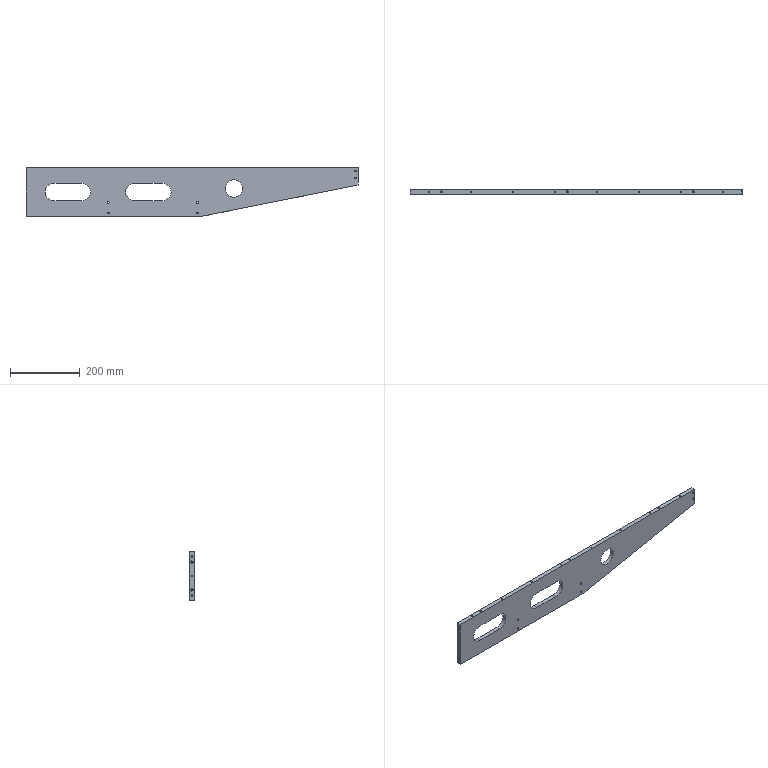Part | SolidWorks | features HoleWzd 8, ICE 2, Chamfer 1 | 1 solid | 136 faces | box 950 x 12 x 140 mm | volume 1176953 mm3 | cylinder 74 | cone 42 | plane 20 | commonest cylinder face diameters 4.2 x16 5.5 x12 10 x12 6 x10 3.3 x8 5 x8